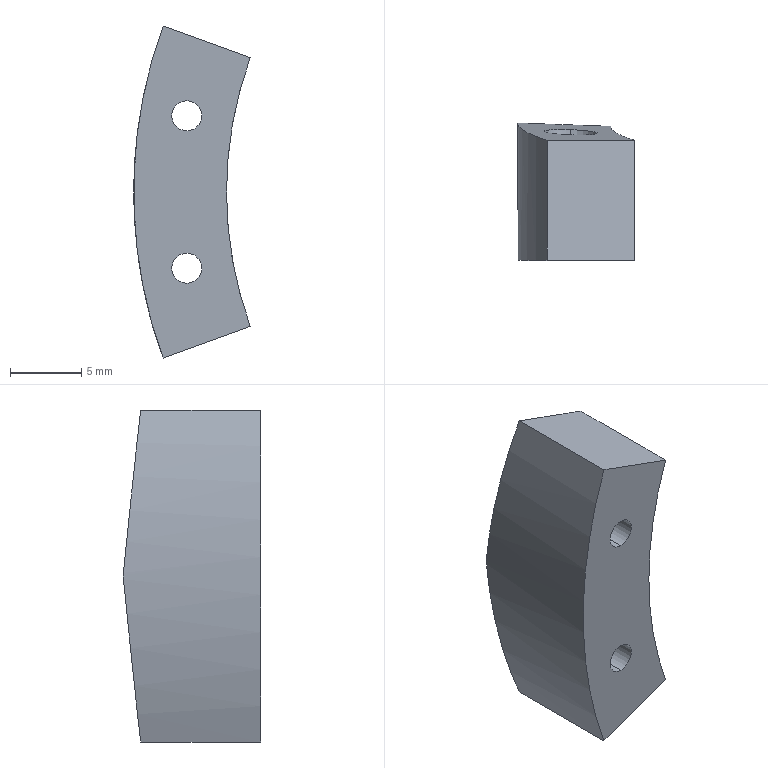Part | SolidWorks | features Chamfer 2, Extrusion 1, ICE 1 | 1 solid | 18 faces | box 8.158 x 9.6 x 23.257 mm | volume 1128 mm3 | cylinder 10 | plane 8 | commonest cylinder face diameters 2.1 x4 3.75 x4 55 x1 68 x1
STEP:
#1=CARTESIAN_POINT('',(-30.283,5.,3.465));
#2=VERTEX_POINT('',#1);
#3=CARTESIAN_POINT('',(-30.283,5.,7.215));
#4=VERTEX_POINT('',#3);
#5=CARTESIAN_POINT('',(-30.283,5.,5.34));
#6=DIRECTION('',(0.,1.,0.));
#7=DIRECTION('',(0.,0.,1.));
#8=AXIS2_PLACEMENT_3D('',#5,#6,#7);
#9=CIRCLE('',#8,1.875);
#10=EDGE_CURVE('',#2,#4,#9,.T.);
#11=ORIENTED_EDGE('',*,*,#10,.F.);
#12=CARTESIAN_POINT('',(-30.283,9.146,3.465));
#13=VERTEX_POINT('',#12);
#14=CARTESIAN_POINT('',(-30.283,-12.308,3.465));
#15=DIRECTION('',(0.,1.,0.));
#16=VECTOR('',#15,1000.);
#17=LINE('',#14,#16);
#18=EDGE_CURVE('',#2,#13,#17,.T.);
#19=ORIENTED_EDGE('',*,*,#18,.T.);
#20=CARTESIAN_POINT('',(-30.283,8.776,7.215));
#21=VERTEX_POINT('',#20);
#22=CARTESIAN_POINT('',(-30.283,8.776,7.215));
#23=CARTESIAN_POINT('',(-33.334,8.886,7.215));
#24=CARTESIAN_POINT('',(-33.229,9.158,4.417));
#25=CARTESIAN_POINT('',(-30.924,9.158,3.578));
#26=CARTESIAN_POINT('',(-30.729,9.158,3.507));
#27=CARTESIAN_POINT('',(-30.513,9.155,3.465));
#28=CARTESIAN_POINT('',(-30.283,9.146,3.465));
#29=(BOUNDED_CURVE()B_SPLINE_CURVE(3,(#22,#23,#24,#25,#26,#27,#28),.UNSPECIFIED.,.F.,.F.)B_SPLINE_CURVE_WITH_KNOTS((4,3,4),(0.07495,0.5,0.5749),.UNSPECIFIED.)CURVE()GEOMETRIC_REPRESENTATION_ITEM()RATIONAL_B_SPLINE_CURVE((0.7451,0.3483,0.4333,1.,0.9001,0.8151,0.7451))REPRESENTATION_ITEM(''));
#30=EDGE_CURVE('',#21,#13,#29,.T.);
#31=ORIENTED_EDGE('',*,*,#30,.F.);
#32=CARTESIAN_POINT('',(-30.283,-12.308,7.215));
#33=DIRECTION('',(0.,1.,0.));
#34=VECTOR('',#33,1000.);
#35=LINE('',#32,#34);
#36=EDGE_CURVE('',#4,#21,#35,.T.);
#37=ORIENTED_EDGE('',*,*,#36,.F.);
#38=EDGE_LOOP('',(#11,#19,#31,#37));
#39=FACE_OUTER_BOUND('',#38,.T.);
#40=CARTESIAN_POINT('',(-30.283,-12.308,5.34));
#41=DIRECTION('',(0.,1.,0.));
#42=DIRECTION('',(0.,0.,1.));
#43=AXIS2_PLACEMENT_3D('',#40,#41,#42);
#44=CYLINDRICAL_SURFACE('',#43,1.875);
#45=ADVANCED_FACE('',(#39),#44,.F.);
#46=CARTESIAN_POINT('',(-30.283,5.,-7.215));
#47=VERTEX_POINT('',#46);
#48=CARTESIAN_POINT('',(-30.283,5.,-3.465));
#49=VERTEX_POINT('',#48);
#50=CARTESIAN_POINT('',(-30.283,5.,-5.34));
#51=DIRECTION('',(0.,1.,0.));
#52=DIRECTION('',(0.,0.,1.));
#53=AXIS2_PLACEMENT_3D('',#50,#51,#52);
#54=CIRCLE('',#53,1.875);
#55=EDGE_CURVE('',#47,#49,#54,.T.);
#56=ORIENTED_EDGE('',*,*,#55,.F.);
#57=CARTESIAN_POINT('',(-30.283,8.776,-7.215));
#58=VERTEX_POINT('',#57);
#59=CARTESIAN_POINT('',(-30.283,-11.253,-7.215));
#60=DIRECTION('',(0.,1.,0.));
#61=VECTOR('',#60,1000.);
#62=LINE('',#59,#61);
#63=EDGE_CURVE('',#47,#58,#62,.T.);
#64=ORIENTED_EDGE('',*,*,#63,.T.);
#65=CARTESIAN_POINT('',(-30.283,9.146,-3.465));
#66=VERTEX_POINT('',#65);
#67=CARTESIAN_POINT('',(-30.283,9.146,-3.465));
#68=CARTESIAN_POINT('',(-34.033,9.281,-3.465));
#69=CARTESIAN_POINT('',(-34.033,8.911,-7.215));
#70=CARTESIAN_POINT('',(-30.283,8.776,-7.215));
#71=(BOUNDED_CURVE()B_SPLINE_CURVE(3,(#67,#68,#69,#70),.UNSPECIFIED.,.F.,.F.)B_SPLINE_CURVE_WITH_KNOTS((4,4),(5.934,9.076),.UNSPECIFIED.)CURVE()GEOMETRIC_REPRESENTATION_ITEM()RATIONAL_B_SPLINE_CURVE((1.,0.3333,0.3333,1.))REPRESENTATION_ITEM(''));
#72=EDGE_CURVE('',#66,#58,#71,.T.);
#73=ORIENTED_EDGE('',*,*,#72,.F.);
#74=CARTESIAN_POINT('',(-30.283,-11.253,-3.465));
#75=DIRECTION('',(0.,1.,0.));
#76=VECTOR('',#75,1000.);
#77=LINE('',#74,#76);
#78=EDGE_CURVE('',#49,#66,#77,.T.);
#79=ORIENTED_EDGE('',*,*,#78,.F.);
#80=EDGE_LOOP('',(#56,#64,#73,#79));
#81=FACE_OUTER_BOUND('',#80,.T.);
#82=CARTESIAN_POINT('',(-30.283,-11.253,-5.34));
#83=DIRECTION('',(0.,1.,0.));
#84=DIRECTION('',(0.,0.,1.));
#85=AXIS2_PLACEMENT_3D('',#82,#83,#84);
#86=CYLINDRICAL_SURFACE('',#85,1.875);
#87=ADVANCED_FACE('',(#81),#86,.F.);
#88=CARTESIAN_POINT('',(-30.283,5.,6.39));
#89=VERTEX_POINT('',#88);
#90=CARTESIAN_POINT('',(-30.283,5.,4.29));
#91=VERTEX_POINT('',#90);
#92=CARTESIAN_POINT('',(-30.283,5.,5.34));
#93=DIRECTION('',(0.,-1.,0.));
#94=DIRECTION('',(0.,0.,1.));
#95=AXIS2_PLACEMENT_3D('',#92,#93,#94);
#96=CIRCLE('',#95,1.05);
#97=EDGE_CURVE('',#89,#91,#96,.T.);
#98=ORIENTED_EDGE('',*,*,#97,.F.);
#99=CARTESIAN_POINT('',(-30.283,0.,6.39));
#100=VERTEX_POINT('',#99);
#101=CARTESIAN_POINT('',(-30.283,9.6,6.39));
#102=DIRECTION('',(0.,-1.,0.));
#103=VECTOR('',#102,1000.);
#104=LINE('',#101,#103);
#105=EDGE_CURVE('',#89,#100,#104,.T.);
#106=ORIENTED_EDGE('',*,*,#105,.T.);
#107=CARTESIAN_POINT('',(-30.283,0.,4.29));
#108=VERTEX_POINT('',#107);
#109=CARTESIAN_POINT('',(-30.283,0.,5.34));
#110=DIRECTION('',(0.,-1.,0.));
#111=DIRECTION('',(0.,0.,1.));
#112=AXIS2_PLACEMENT_3D('',#109,#110,#111);
#113=CIRCLE('',#112,1.05);
#114=EDGE_CURVE('',#100,#108,#113,.T.);
#115=ORIENTED_EDGE('',*,*,#114,.T.);
#116=CARTESIAN_POINT('',(-30.283,9.6,4.29));
#117=DIRECTION('',(0.,-1.,0.));
#118=VECTOR('',#117,1000.);
#119=LINE('',#116,#118);
#120=EDGE_CURVE('',#91,#108,#119,.T.);
#121=ORIENTED_EDGE('',*,*,#120,.F.);
#122=EDGE_LOOP('',(#98,#106,#115,#121));
#123=FACE_OUTER_BOUND('',#122,.T.);
#124=CARTESIAN_POINT('',(-30.283,9.6,5.34));
#125=DIRECTION('',(0.,-1.,0.));
#126=DIRECTION('',(0.,0.,-1.));
#127=AXIS2_PLACEMENT_3D('',#124,#125,#126);
#128=CYLINDRICAL_SURFACE('',#127,1.05);
#129=ADVANCED_FACE('',(#123),#128,.F.);
#130=CARTESIAN_POINT('',(-30.283,5.,-6.39));
#131=VERTEX_POINT('',#130);
#132=CARTESIAN_POINT('',(-30.283,5.,-4.29));
#133=VERTEX_POINT('',#132);
#134=CARTESIAN_POINT('',(-30.283,5.,-5.34));
#135=DIRECTION('',(0.,1.,0.));
#136=DIRECTION('',(0.,0.,1.));
#137=AXIS2_PLACEMENT_3D('',#134,#135,#136);
#138=CIRCLE('',#137,1.05);
#139=EDGE_CURVE('',#131,#133,#138,.T.);
#140=ORIENTED_EDGE('',*,*,#139,.T.);
#141=CARTESIAN_POINT('',(-30.283,0.,-4.29));
#142=VERTEX_POINT('',#141);
#143=CARTESIAN_POINT('',(-30.283,9.6,-4.29));
#144=DIRECTION('',(0.,-1.,0.));
#145=VECTOR('',#144,1000.);
#146=LINE('',#143,#145);
#147=EDGE_CURVE('',#133,#142,#146,.T.);
#148=ORIENTED_EDGE('',*,*,#147,.T.);
#149=CARTESIAN_POINT('',(-30.283,0.,-6.39));
#150=VERTEX_POINT('',#149);
#151=CARTESIAN_POINT('',(-30.283,0.,-5.34));
#152=DIRECTION('',(0.,1.,0.));
#153=DIRECTION('',(0.,0.,1.));
#154=AXIS2_PLACEMENT_3D('',#151,#152,#153);
#155=CIRCLE('',#154,1.05);
#156=EDGE_CURVE('',#150,#142,#155,.T.);
#157=ORIENTED_EDGE('',*,*,#156,.F.);
#158=CARTESIAN_POINT('',(-30.283,9.6,-6.39));
#159=DIRECTION('',(0.,-1.,0.));
#160=VECTOR('',#159,1000.);
#161=LINE('',#158,#160);
#162=EDGE_CURVE('',#131,#150,#161,.T.);
#163=ORIENTED_EDGE('',*,*,#162,.F.);
#164=EDGE_LOOP('',(#140,#148,#157,#163));
#165=FACE_OUTER_BOUND('',#164,.T.);
#166=CARTESIAN_POINT('',(-30.283,9.6,-5.34));
#167=DIRECTION('',(0.,-1.,0.));
#168=DIRECTION('',(0.,0.,-1.));
#169=AXIS2_PLACEMENT_3D('',#166,#167,#168);
#170=CYLINDRICAL_SURFACE('',#169,1.05);
#171=ADVANCED_FACE('',(#165),#170,.F.);
#172=ORIENTED_EDGE('',*,*,#147,.F.);
#173=CARTESIAN_POINT('',(-30.283,5.,-5.34));
#174=DIRECTION('',(0.,1.,0.));
#175=DIRECTION('',(0.,0.,1.));
#176=AXIS2_PLACEMENT_3D('',#173,#174,#175);
#177=CIRCLE('',#176,1.05);
#178=EDGE_CURVE('',#133,#131,#177,.T.);
#179=ORIENTED_EDGE('',*,*,#178,.T.);
#180=ORIENTED_EDGE('',*,*,#162,.T.);
#181=CARTESIAN_POINT('',(-30.283,0.,-5.34));
#182=DIRECTION('',(0.,1.,0.));
#183=DIRECTION('',(0.,0.,1.));
#184=AXIS2_PLACEMENT_3D('',#181,#182,#183);
#185=CIRCLE('',#184,1.05);
#186=EDGE_CURVE('',#142,#150,#185,.T.);
#187=ORIENTED_EDGE('',*,*,#186,.F.);
#188=EDGE_LOOP('',(#172,#179,#180,#187));
#189=FACE_OUTER_BOUND('',#188,.T.);
#190=CARTESIAN_POINT('',(-30.283,9.6,-5.34));
#191=DIRECTION('',(0.,-1.,0.));
#192=DIRECTION('',(0.,0.,-1.));
#193=AXIS2_PLACEMENT_3D('',#190,#191,#192);
#194=CYLINDRICAL_SURFACE('',#193,1.05);
#195=ADVANCED_FACE('',(#189),#194,.F.);
#196=ORIENTED_EDGE('',*,*,#105,.F.);
#197=CARTESIAN_POINT('',(-30.283,5.,5.34));
#198=DIRECTION('',(0.,-1.,0.));
#199=DIRECTION('',(0.,0.,1.));
#200=AXIS2_PLACEMENT_3D('',#197,#198,#199);
#201=CIRCLE('',#200,1.05);
#202=EDGE_CURVE('',#91,#89,#201,.T.);
#203=ORIENTED_EDGE('',*,*,#202,.F.);
#204=ORIENTED_EDGE('',*,*,#120,.T.);
#205=CARTESIAN_POINT('',(-30.283,0.,5.34));
#206=DIRECTION('',(0.,-1.,0.));
#207=DIRECTION('',(0.,0.,1.));
#208=AXIS2_PLACEMENT_3D('',#205,#206,#207);
#209=CIRCLE('',#208,1.05);
#210=EDGE_CURVE('',#108,#100,#209,.T.);
#211=ORIENTED_EDGE('',*,*,#210,.T.);
#212=EDGE_LOOP('',(#196,#203,#204,#211));
#213=FACE_OUTER_BOUND('',#212,.T.);
#214=CARTESIAN_POINT('',(-30.283,9.6,5.34));
#215=DIRECTION('',(0.,-1.,0.));
#216=DIRECTION('',(0.,0.,-1.));
#217=AXIS2_PLACEMENT_3D('',#214,#215,#216);
#218=CYLINDRICAL_SURFACE('',#217,1.05);
#219=ADVANCED_FACE('',(#213),#218,.F.);
#220=CARTESIAN_POINT('',(-31.95,8.4,-11.629));
#221=VERTEX_POINT('',#220);
#222=CARTESIAN_POINT('',(-31.95,0.,-11.629));
#223=VERTEX_POINT('',#222);
#224=CARTESIAN_POINT('',(-31.95,9.6,-11.629));
#225=DIRECTION('',(0.,-1.,0.));
#226=VECTOR('',#225,1000.);
#227=LINE('',#224,#226);
#228=EDGE_CURVE('',#221,#223,#227,.T.);
#229=ORIENTED_EDGE('',*,*,#228,.F.);
#230=CARTESIAN_POINT('',(-25.842,8.4,-9.406));
#231=VERTEX_POINT('',#230);
#232=CARTESIAN_POINT('',(-25.842,8.4,-9.406));
#233=DIRECTION('',(0.9397,0.,0.342));
#234=VECTOR('',#233,1000.);
#235=LINE('',#232,#234);
#236=EDGE_CURVE('',#221,#231,#235,.T.);
#237=ORIENTED_EDGE('',*,*,#236,.T.);
#238=CARTESIAN_POINT('',(-25.842,0.,-9.406));
#239=VERTEX_POINT('',#238);
#240=CARTESIAN_POINT('',(-25.842,9.6,-9.406));
#241=DIRECTION('',(0.,-1.,0.));
#242=VECTOR('',#241,1000.);
#243=LINE('',#240,#242);
#244=EDGE_CURVE('',#231,#239,#243,.T.);
#245=ORIENTED_EDGE('',*,*,#244,.T.);
#246=CARTESIAN_POINT('',(0.,0.,0.));
#247=DIRECTION('',(-0.9397,0.,-0.342));
#248=VECTOR('',#247,1000.);
#249=LINE('',#246,#248);
#250=EDGE_CURVE('',#239,#223,#249,.T.);
#251=ORIENTED_EDGE('',*,*,#250,.T.);
#252=EDGE_LOOP('',(#229,#237,#245,#251));
#253=FACE_OUTER_BOUND('',#252,.T.);
#254=CARTESIAN_POINT('',(0.,9.6,0.));
#255=DIRECTION('',(-0.342,0.,0.9397));
#256=DIRECTION('',(0.9397,0.,0.342));
#257=AXIS2_PLACEMENT_3D('',#254,#255,#256);
#258=PLANE('',#257);
#259=ADVANCED_FACE('',(#253),#258,.F.);
#260=CARTESIAN_POINT('',(-33.999,9.6,-0.2247));
#261=VERTEX_POINT('',#260);
#262=CARTESIAN_POINT('',(-33.999,9.6,0.2247));
#263=VERTEX_POINT('',#262);
#264=CARTESIAN_POINT('',(0.,9.6,0.));
#265=DIRECTION('',(0.,1.,0.));
#266=DIRECTION('',(0.,0.,1.));
#267=AXIS2_PLACEMENT_3D('',#264,#265,#266);
#268=CIRCLE('',#267,34.);
#269=EDGE_CURVE('',#261,#263,#268,.T.);
#270=ORIENTED_EDGE('',*,*,#269,.F.);
#271=CARTESIAN_POINT('',(-33.999,9.6,-0.2247));
#272=CARTESIAN_POINT('',(-33.973,9.214,-4.125));
#273=CARTESIAN_POINT('',(-33.284,8.81,-7.964));
#274=CARTESIAN_POINT('',(-31.95,8.4,-11.629));
#275=(BOUNDED_CURVE()B_SPLINE_CURVE(3,(#271,#272,#273,#274),.UNSPECIFIED.,.F.,.F.)B_SPLINE_CURVE_WITH_KNOTS((4,4),(4.37,4.712),.UNSPECIFIED.)CURVE()GEOMETRIC_REPRESENTATION_ITEM()RATIONAL_B_SPLINE_CURVE((1.,0.9903,0.9903,1.))REPRESENTATION_ITEM(''));
#276=EDGE_CURVE('',#261,#221,#275,.T.);
#277=ORIENTED_EDGE('',*,*,#276,.T.);
#278=ORIENTED_EDGE('',*,*,#228,.T.);
#279=CARTESIAN_POINT('',(-31.95,0.,11.629));
#280=VERTEX_POINT('',#279);
#281=CARTESIAN_POINT('',(0.,0.,0.));
#282=DIRECTION('',(0.,1.,0.));
#283=DIRECTION('',(0.,0.,1.));
#284=AXIS2_PLACEMENT_3D('',#281,#282,#283);
#285=CIRCLE('',#284,34.);
#286=EDGE_CURVE('',#223,#280,#285,.T.);
#287=ORIENTED_EDGE('',*,*,#286,.T.);
#288=CARTESIAN_POINT('',(-31.95,8.4,11.629));
#289=VERTEX_POINT('',#288);
#290=CARTESIAN_POINT('',(-31.95,9.6,11.629));
#291=DIRECTION('',(0.,-1.,0.));
#292=VECTOR('',#291,1000.);
#293=LINE('',#290,#292);
#294=EDGE_CURVE('',#289,#280,#293,.T.);
#295=ORIENTED_EDGE('',*,*,#294,.F.);
#296=CARTESIAN_POINT('',(-31.95,8.4,11.629));
#297=CARTESIAN_POINT('',(-33.284,8.81,7.964));
#298=CARTESIAN_POINT('',(-33.973,9.214,4.125));
#299=CARTESIAN_POINT('',(-33.999,9.6,0.2247));
#300=(BOUNDED_CURVE()B_SPLINE_CURVE(3,(#296,#297,#298,#299),.UNSPECIFIED.,.F.,.F.)B_SPLINE_CURVE_WITH_KNOTS((4,4),(1.571,1.913),.UNSPECIFIED.)CURVE()GEOMETRIC_REPRESENTATION_ITEM()RATIONAL_B_SPLINE_CURVE((1.,0.9903,0.9903,1.))REPRESENTATION_ITEM(''));
#301=EDGE_CURVE('',#289,#263,#300,.T.);
#302=ORIENTED_EDGE('',*,*,#301,.T.);
#303=EDGE_LOOP('',(#270,#277,#278,#287,#295,#302));
#304=FACE_OUTER_BOUND('',#303,.T.);
#305=CARTESIAN_POINT('',(0.,9.6,0.));
#306=DIRECTION('',(0.,-1.,0.));
#307=DIRECTION('',(0.,0.,-1.));
#308=AXIS2_PLACEMENT_3D('',#305,#306,#307);
#309=CYLINDRICAL_SURFACE('',#308,34.);
#310=ADVANCED_FACE('',(#304),#309,.T.);
#311=CARTESIAN_POINT('',(-25.842,8.4,9.406));
#312=VERTEX_POINT('',#311);
#313=CARTESIAN_POINT('',(-25.842,0.,9.406));
#314=VERTEX_POINT('',#313);
#315=CARTESIAN_POINT('',(-25.842,9.6,9.406));
#316=DIRECTION('',(0.,-1.,0.));
#317=VECTOR('',#316,1000.);
#318=LINE('',#315,#317);
#319=EDGE_CURVE('',#312,#314,#318,.T.);
#320=ORIENTED_EDGE('',*,*,#319,.F.);
#321=CARTESIAN_POINT('',(0.,8.4,0.));
#322=DIRECTION('',(-0.9397,0.,0.342));
#323=VECTOR('',#322,1000.);
#324=LINE('',#321,#323);
#325=EDGE_CURVE('',#312,#289,#324,.T.);
#326=ORIENTED_EDGE('',*,*,#325,.T.);
#327=ORIENTED_EDGE('',*,*,#294,.T.);
#328=CARTESIAN_POINT('',(0.,0.,0.));
#329=DIRECTION('',(-0.9397,0.,0.342));
#330=VECTOR('',#329,1000.);
#331=LINE('',#328,#330);
#332=EDGE_CURVE('',#314,#280,#331,.T.);
#333=ORIENTED_EDGE('',*,*,#332,.F.);
#334=EDGE_LOOP('',(#320,#326,#327,#333));
#335=FACE_OUTER_BOUND('',#334,.T.);
#336=CARTESIAN_POINT('',(0.,9.6,0.));
#337=DIRECTION('',(0.342,0.,0.9397));
#338=DIRECTION('',(0.9397,0.,-0.342));
#339=AXIS2_PLACEMENT_3D('',#336,#337,#338);
#340=PLANE('',#339);
#341=ADVANCED_FACE('',(#335),#340,.T.);
#342=ORIENTED_EDGE('',*,*,#244,.F.);
#343=CARTESIAN_POINT('',(-27.5,9.389,0.));
#344=VERTEX_POINT('',#343);
#345=CARTESIAN_POINT('',(-25.842,8.4,-9.406));
#346=CARTESIAN_POINT('',(-26.942,8.738,-6.383));
#347=CARTESIAN_POINT('',(-27.5,9.071,-3.216));
#348=CARTESIAN_POINT('',(-27.5,9.389,0.));
#349=(BOUNDED_CURVE()B_SPLINE_CURVE(3,(#345,#346,#347,#348),.UNSPECIFIED.,.F.,.F.)B_SPLINE_CURVE_WITH_KNOTS((4,4),(1.571,1.92),.UNSPECIFIED.)CURVE()GEOMETRIC_REPRESENTATION_ITEM()RATIONAL_B_SPLINE_CURVE((1.,0.9899,0.9899,1.))REPRESENTATION_ITEM(''));
#350=EDGE_CURVE('',#231,#344,#349,.T.);
#351=ORIENTED_EDGE('',*,*,#350,.T.);
#352=CARTESIAN_POINT('',(-27.5,9.389,0.));
#353=CARTESIAN_POINT('',(-27.5,9.071,3.216));
#354=CARTESIAN_POINT('',(-26.942,8.738,6.383));
#355=CARTESIAN_POINT('',(-25.842,8.4,9.406));
#356=(BOUNDED_CURVE()B_SPLINE_CURVE(3,(#352,#353,#354,#355),.UNSPECIFIED.,.F.,.F.)B_SPLINE_CURVE_WITH_KNOTS((4,4),(4.363,4.712),.UNSPECIFIED.)CURVE()GEOMETRIC_REPRESENTATION_ITEM()RATIONAL_B_SPLINE_CURVE((1.,0.9899,0.9899,1.))REPRESENTATION_ITEM(''));
#357=EDGE_CURVE('',#344,#312,#356,.T.);
#358=ORIENTED_EDGE('',*,*,#357,.T.);
#359=ORIENTED_EDGE('',*,*,#319,.T.);
#360=CARTESIAN_POINT('',(0.,0.,0.));
#361=DIRECTION('',(0.,1.,0.));
#362=DIRECTION('',(0.,0.,1.));
#363=AXIS2_PLACEMENT_3D('',#360,#361,#362);
#364=CIRCLE('',#363,27.5);
#365=EDGE_CURVE('',#239,#314,#364,.T.);
#366=ORIENTED_EDGE('',*,*,#365,.F.);
#367=EDGE_LOOP('',(#342,#351,#358,#359,#366));
#368=FACE_OUTER_BOUND('',#367,.T.);
#369=CARTESIAN_POINT('',(0.,9.6,0.));
#370=DIRECTION('',(0.,-1.,0.));
#371=DIRECTION('',(0.,0.,-1.));
#372=AXIS2_PLACEMENT_3D('',#369,#370,#371);
#373=CYLINDRICAL_SURFACE('',#372,27.5);
#374=ADVANCED_FACE('',(#368),#373,.F.);
#375=CARTESIAN_POINT('',(-33.382,9.6,0.));
#376=VERTEX_POINT('',#375);
#377=CARTESIAN_POINT('',(-3.905,9.6,-10.729));
#378=DIRECTION('',(0.9397,0.,-0.342));
#379=VECTOR('',#378,1000.);
#380=LINE('',#377,#379);
#381=EDGE_CURVE('',#263,#376,#380,.T.);
#382=ORIENTED_EDGE('',*,*,#381,.T.);
#383=CARTESIAN_POINT('',(-35.854,9.6,-0.9));
#384=DIRECTION('',(-0.9397,0.,-0.342));
#385=VECTOR('',#384,1000.);
#386=LINE('',#383,#385);
#387=EDGE_CURVE('',#376,#261,#386,.T.);
#388=ORIENTED_EDGE('',*,*,#387,.T.);
#389=ORIENTED_EDGE('',*,*,#269,.T.);
#390=EDGE_LOOP('',(#382,#388,#389));
#391=FACE_OUTER_BOUND('',#390,.T.);
#392=CARTESIAN_POINT('',(0.,9.6,0.));
#393=DIRECTION('',(0.,1.,0.));
#394=DIRECTION('',(0.,0.,1.));
#395=AXIS2_PLACEMENT_3D('',#392,#393,#394);
#396=PLANE('',#395);
#397=ADVANCED_FACE('',(#391),#396,.T.);
#398=ORIENTED_EDGE('',*,*,#250,.F.);
#399=ORIENTED_EDGE('',*,*,#365,.T.);
#400=ORIENTED_EDGE('',*,*,#332,.T.);
#401=ORIENTED_EDGE('',*,*,#286,.F.);
#402=EDGE_LOOP('',(#398,#399,#400,#401));
#403=FACE_OUTER_BOUND('',#402,.T.);
#404=ORIENTED_EDGE('',*,*,#156,.T.);
#405=ORIENTED_EDGE('',*,*,#186,.T.);
#406=EDGE_LOOP('',(#404,#405));
#407=FACE_BOUND('',#406,.T.);
#408=ORIENTED_EDGE('',*,*,#210,.F.);
#409=ORIENTED_EDGE('',*,*,#114,.F.);
#410=EDGE_LOOP('',(#408,#409));
#411=FACE_BOUND('',#410,.T.);
#412=CARTESIAN_POINT('',(0.,0.,0.));
#413=DIRECTION('',(0.,1.,0.));
#414=DIRECTION('',(0.,0.,1.));
#415=AXIS2_PLACEMENT_3D('',#412,#413,#414);
#416=PLANE('',#415);
#417=ADVANCED_FACE('',(#403,#407,#411),#416,.F.);
#418=ORIENTED_EDGE('',*,*,#30,.T.);
#419=CARTESIAN_POINT('',(-30.283,9.146,3.465));
#420=CARTESIAN_POINT('',(-27.232,9.037,3.465));
#421=CARTESIAN_POINT('',(-27.337,8.764,6.263));
#422=CARTESIAN_POINT('',(-29.642,8.764,7.102));
#423=CARTESIAN_POINT('',(-29.837,8.764,7.173));
#424=CARTESIAN_POINT('',(-30.053,8.768,7.215));
#425=CARTESIAN_POINT('',(-30.283,8.776,7.215));
#426=(BOUNDED_CURVE()B_SPLINE_CURVE(3,(#419,#420,#421,#422,#423,#424,#425),.UNSPECIFIED.,.F.,.F.)B_SPLINE_CURVE_WITH_KNOTS((4,3,4),(0.5749,1.,1.075),.UNSPECIFIED.)CURVE()GEOMETRIC_REPRESENTATION_ITEM()RATIONAL_B_SPLINE_CURVE((0.7451,0.3483,0.4333,1.,0.9001,0.8151,0.7451))REPRESENTATION_ITEM(''));
#427=EDGE_CURVE('',#13,#21,#426,.T.);
#428=ORIENTED_EDGE('',*,*,#427,.T.);
#429=EDGE_LOOP('',(#418,#428));
#430=FACE_BOUND('',#429,.T.);
#431=ORIENTED_EDGE('',*,*,#357,.F.);
#432=CARTESIAN_POINT('',(0.,8.4,0.));
#433=DIRECTION('',(-0.9994,0.03592,0.));
#434=VECTOR('',#433,1000.);
#435=LINE('',#432,#434);
#436=EDGE_CURVE('',#344,#376,#435,.T.);
#437=ORIENTED_EDGE('',*,*,#436,.T.);
#438=ORIENTED_EDGE('',*,*,#381,.F.);
#439=ORIENTED_EDGE('',*,*,#301,.F.);
#440=ORIENTED_EDGE('',*,*,#325,.F.);
#441=EDGE_LOOP('',(#431,#437,#438,#439,#440));
#442=FACE_OUTER_BOUND('',#441,.T.);
#443=CARTESIAN_POINT('',(0.,8.4,0.));
#444=DIRECTION('',(-0.03575,-0.9945,-0.09822));
#445=DIRECTION('',(-0.9397,0.,0.342));
#446=AXIS2_PLACEMENT_3D('',#443,#444,#445);
#447=PLANE('',#446);
#448=ADVANCED_FACE('',(#430,#442),#447,.F.);
#449=ORIENTED_EDGE('',*,*,#72,.T.);
#450=CARTESIAN_POINT('',(-30.283,8.776,-7.215));
#451=CARTESIAN_POINT('',(-26.533,8.641,-7.215));
#452=CARTESIAN_POINT('',(-26.533,9.012,-3.465));
#453=CARTESIAN_POINT('',(-30.283,9.146,-3.465));
#454=(BOUNDED_CURVE()B_SPLINE_CURVE(3,(#450,#451,#452,#453),.UNSPECIFIED.,.F.,.F.)B_SPLINE_CURVE_WITH_KNOTS((4,4),(2.793,5.934),.UNSPECIFIED.)CURVE()GEOMETRIC_REPRESENTATION_ITEM()RATIONAL_B_SPLINE_CURVE((1.,0.3333,0.3333,1.))REPRESENTATION_ITEM(''));
#455=EDGE_CURVE('',#58,#66,#454,.T.);
#456=ORIENTED_EDGE('',*,*,#455,.T.);
#457=EDGE_LOOP('',(#449,#456));
#458=FACE_BOUND('',#457,.T.);
#459=ORIENTED_EDGE('',*,*,#350,.F.);
#460=ORIENTED_EDGE('',*,*,#236,.F.);
#461=ORIENTED_EDGE('',*,*,#276,.F.);
#462=ORIENTED_EDGE('',*,*,#387,.F.);
#463=ORIENTED_EDGE('',*,*,#436,.F.);
#464=EDGE_LOOP('',(#459,#460,#461,#462,#463));
#465=FACE_OUTER_BOUND('',#464,.T.);
#466=CARTESIAN_POINT('',(-3.905,9.6,10.729));
#467=DIRECTION('',(0.03575,0.9945,-0.09822));
#468=DIRECTION('',(0.9397,0.,0.342));
#469=AXIS2_PLACEMENT_3D('',#466,#467,#468);
#470=PLANE('',#469);
#471=ADVANCED_FACE('',(#458,#465),#470,.T.);
#472=ORIENTED_EDGE('',*,*,#63,.F.);
#473=CARTESIAN_POINT('',(-30.283,5.,-5.34));
#474=DIRECTION('',(0.,1.,0.));
#475=DIRECTION('',(0.,0.,1.));
#476=AXIS2_PLACEMENT_3D('',#473,#474,#475);
#477=CIRCLE('',#476,1.875);
#478=EDGE_CURVE('',#49,#47,#477,.T.);
#479=ORIENTED_EDGE('',*,*,#478,.F.);
#480=ORIENTED_EDGE('',*,*,#78,.T.);
#481=ORIENTED_EDGE('',*,*,#455,.F.);
#482=EDGE_LOOP('',(#472,#479,#480,#481));
#483=FACE_OUTER_BOUND('',#482,.T.);
#484=CARTESIAN_POINT('',(-30.283,-11.253,-5.34));
#485=DIRECTION('',(0.,1.,0.));
#486=DIRECTION('',(0.,0.,1.));
#487=AXIS2_PLACEMENT_3D('',#484,#485,#486);
#488=CYLINDRICAL_SURFACE('',#487,1.875);
#489=ADVANCED_FACE('',(#483),#488,.F.);
#490=ORIENTED_EDGE('',*,*,#139,.F.);
#491=ORIENTED_EDGE('',*,*,#178,.F.);
#492=EDGE_LOOP('',(#490,#491));
#493=FACE_BOUND('',#492,.T.);
#494=ORIENTED_EDGE('',*,*,#478,.T.);
#495=ORIENTED_EDGE('',*,*,#55,.T.);
#496=EDGE_LOOP('',(#494,#495));
#497=FACE_OUTER_BOUND('',#496,.T.);
#498=CARTESIAN_POINT('',(0.,5.,0.));
#499=DIRECTION('',(0.,1.,0.));
#500=DIRECTION('',(0.,0.,1.));
#501=AXIS2_PLACEMENT_3D('',#498,#499,#500);
#502=PLANE('',#501);
#503=ADVANCED_FACE('',(#493,#497),#502,.T.);
#504=CARTESIAN_POINT('',(-30.283,5.,5.34));
#505=DIRECTION('',(0.,1.,0.));
#506=DIRECTION('',(0.,0.,1.));
#507=AXIS2_PLACEMENT_3D('',#504,#505,#506);
#508=CIRCLE('',#507,1.875);
#509=EDGE_CURVE('',#4,#2,#508,.T.);
#510=ORIENTED_EDGE('',*,*,#509,.T.);
#511=ORIENTED_EDGE('',*,*,#10,.T.);
#512=EDGE_LOOP('',(#510,#511));
#513=FACE_OUTER_BOUND('',#512,.T.);
#514=ORIENTED_EDGE('',*,*,#202,.T.);
#515=ORIENTED_EDGE('',*,*,#97,.T.);
#516=EDGE_LOOP('',(#514,#515));
#517=FACE_BOUND('',#516,.T.);
#518=CARTESIAN_POINT('',(0.,5.,0.));
#519=DIRECTION('',(0.,1.,0.));
#520=DIRECTION('',(0.,0.,1.));
#521=AXIS2_PLACEMENT_3D('',#518,#519,#520);
#522=PLANE('',#521);
#523=ADVANCED_FACE('',(#513,#517),#522,.T.);
#524=ORIENTED_EDGE('',*,*,#18,.F.);
#525=ORIENTED_EDGE('',*,*,#509,.F.);
#526=ORIENTED_EDGE('',*,*,#36,.T.);
#527=ORIENTED_EDGE('',*,*,#427,.F.);
#528=EDGE_LOOP('',(#524,#525,#526,#527));
#529=FACE_OUTER_BOUND('',#528,.T.);
#530=CARTESIAN_POINT('',(-30.283,-12.308,5.34));
#531=DIRECTION('',(0.,1.,0.));
#532=DIRECTION('',(0.,0.,1.));
#533=AXIS2_PLACEMENT_3D('',#530,#531,#532);
#534=CYLINDRICAL_SURFACE('',#533,1.875);
#535=ADVANCED_FACE('',(#529),#534,.F.);
#536=CLOSED_SHELL('',(#45,#87,#129,#171,#195,#219,#259,#310,#341,#374,#397,#417,#448,#471,#489,#503,#523,#535));
#537=MANIFOLD_SOLID_BREP('',#536);
#538=CARTESIAN_POINT('',(0.,0.,0.));
#539=DIRECTION('',(0.,0.,1.));
#540=DIRECTION('',(1.,0.,0.));
#541=AXIS2_PLACEMENT_3D('',#538,#539,#540);
#542=(LENGTH_UNIT()NAMED_UNIT(*)SI_UNIT(.MILLI.,.METRE.));
#543=UNCERTAINTY_MEASURE_WITH_UNIT(LENGTH_MEASURE(0.00001),#542,'','');
#544=(NAMED_UNIT(*)PLANE_ANGLE_UNIT()SI_UNIT($,.RADIAN.));
#545=(NAMED_UNIT(*)SI_UNIT($,.STERADIAN.)SOLID_ANGLE_UNIT());
#546=(GEOMETRIC_REPRESENTATION_CONTEXT(3)GLOBAL_UNCERTAINTY_ASSIGNED_CONTEXT((#543))GLOBAL_UNIT_ASSIGNED_CONTEXT((#542,#544,#545))REPRESENTATION_CONTEXT('',''));
#547=ADVANCED_BREP_SHAPE_REPRESENTATION('',(#537,#541),#546);